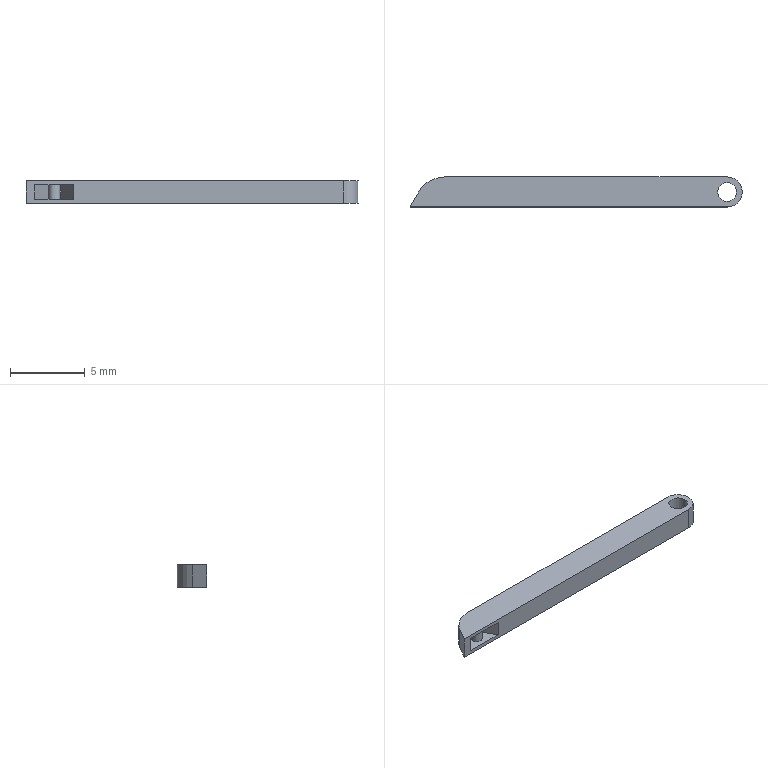Part | SolidWorks | features Extrusion 1, Fillet 1, ICE 1 | 1 solid | 16 faces | box 22.155 x 2 x 1.5 mm | volume 59.83 mm3 | plane 10 | cylinder 6 | commonest cylinder face diameters 0.8 x2 1.25 x2 2 x1 4 x1
STEP:
#1=CARTESIAN_POINT('',(0.3217,-1.25,1.25));
#2=VERTEX_POINT('',#1);
#3=CARTESIAN_POINT('',(1.122,-1.25,1.25));
#4=VERTEX_POINT('',#3);
#5=CARTESIAN_POINT('',(0.7217,-1.25,1.25));
#6=DIRECTION('',(0.,0.,-1.));
#7=DIRECTION('',(-1.,0.,0.));
#8=AXIS2_PLACEMENT_3D('',#5,#6,#7);
#9=CIRCLE('',#8,0.4);
#10=EDGE_CURVE('',#2,#4,#9,.T.);
#11=ORIENTED_EDGE('',*,*,#10,.T.);
#12=CARTESIAN_POINT('',(1.122,-1.25,0.25));
#13=VERTEX_POINT('',#12);
#14=CARTESIAN_POINT('',(1.122,-1.25,1.25));
#15=DIRECTION('',(0.,0.,-1.));
#16=VECTOR('',#15,1000.);
#17=LINE('',#14,#16);
#18=EDGE_CURVE('',#4,#13,#17,.T.);
#19=ORIENTED_EDGE('',*,*,#18,.T.);
#20=CARTESIAN_POINT('',(0.3217,-1.25,0.25));
#21=VERTEX_POINT('',#20);
#22=CARTESIAN_POINT('',(0.7217,-1.25,0.25));
#23=DIRECTION('',(0.,0.,-1.));
#24=DIRECTION('',(-1.,0.,0.));
#25=AXIS2_PLACEMENT_3D('',#22,#23,#24);
#26=CIRCLE('',#25,0.4);
#27=EDGE_CURVE('',#21,#13,#26,.T.);
#28=ORIENTED_EDGE('',*,*,#27,.F.);
#29=CARTESIAN_POINT('',(0.3217,-1.25,1.25));
#30=DIRECTION('',(0.,0.,-1.));
#31=VECTOR('',#30,1000.);
#32=LINE('',#29,#31);
#33=EDGE_CURVE('',#2,#21,#32,.T.);
#34=ORIENTED_EDGE('',*,*,#33,.F.);
#35=EDGE_LOOP('',(#11,#19,#28,#34));
#36=FACE_OUTER_BOUND('',#35,.T.);
#37=CARTESIAN_POINT('',(0.7217,-1.25,1.25));
#38=DIRECTION('',(0.,0.,-1.));
#39=DIRECTION('',(-1.,0.,0.));
#40=AXIS2_PLACEMENT_3D('',#37,#38,#39);
#41=CYLINDRICAL_SURFACE('',#40,0.4);
#42=ADVANCED_FACE('',(#36),#41,.T.);
#43=CARTESIAN_POINT('',(19.375,-1.,1.5));
#44=VERTEX_POINT('',#43);
#45=CARTESIAN_POINT('',(20.625,-1.,1.5));
#46=VERTEX_POINT('',#45);
#47=CARTESIAN_POINT('',(20.,-1.,1.5));
#48=DIRECTION('',(0.,0.,1.));
#49=DIRECTION('',(1.,0.,0.));
#50=AXIS2_PLACEMENT_3D('',#47,#48,#49);
#51=CIRCLE('',#50,0.625);
#52=EDGE_CURVE('',#44,#46,#51,.T.);
#53=ORIENTED_EDGE('',*,*,#52,.T.);
#54=CARTESIAN_POINT('',(20.625,-1.,0.));
#55=VERTEX_POINT('',#54);
#56=CARTESIAN_POINT('',(20.625,-1.,1.5));
#57=DIRECTION('',(0.,0.,-1.));
#58=VECTOR('',#57,1000.);
#59=LINE('',#56,#58);
#60=EDGE_CURVE('',#46,#55,#59,.T.);
#61=ORIENTED_EDGE('',*,*,#60,.T.);
#62=CARTESIAN_POINT('',(19.375,-1.,0.));
#63=VERTEX_POINT('',#62);
#64=CARTESIAN_POINT('',(20.,-1.,0.));
#65=DIRECTION('',(0.,0.,1.));
#66=DIRECTION('',(1.,0.,0.));
#67=AXIS2_PLACEMENT_3D('',#64,#65,#66);
#68=CIRCLE('',#67,0.625);
#69=EDGE_CURVE('',#63,#55,#68,.T.);
#70=ORIENTED_EDGE('',*,*,#69,.F.);
#71=CARTESIAN_POINT('',(19.375,-1.,1.5));
#72=DIRECTION('',(0.,0.,-1.));
#73=VECTOR('',#72,1000.);
#74=LINE('',#71,#73);
#75=EDGE_CURVE('',#44,#63,#74,.T.);
#76=ORIENTED_EDGE('',*,*,#75,.F.);
#77=EDGE_LOOP('',(#53,#61,#70,#76));
#78=FACE_OUTER_BOUND('',#77,.T.);
#79=CARTESIAN_POINT('',(20.,-1.,1.5));
#80=DIRECTION('',(0.,0.,-1.));
#81=DIRECTION('',(-1.,0.,0.));
#82=AXIS2_PLACEMENT_3D('',#79,#80,#81);
#83=CYLINDRICAL_SURFACE('',#82,0.625);
#84=ADVANCED_FACE('',(#78),#83,.F.);
#85=CARTESIAN_POINT('',(-1.155,-2.,0.));
#86=VERTEX_POINT('',#85);
#87=CARTESIAN_POINT('',(20.,-2.,0.));
#88=VERTEX_POINT('',#87);
#89=CARTESIAN_POINT('',(20.,-2.,0.));
#90=DIRECTION('',(1.,0.,0.));
#91=VECTOR('',#90,1000.);
#92=LINE('',#89,#91);
#93=EDGE_CURVE('',#86,#88,#92,.T.);
#94=ORIENTED_EDGE('',*,*,#93,.T.);
#95=CARTESIAN_POINT('',(20.,-2.,1.5));
#96=VERTEX_POINT('',#95);
#97=CARTESIAN_POINT('',(20.,-2.,1.5));
#98=DIRECTION('',(0.,0.,-1.));
#99=VECTOR('',#98,1000.);
#100=LINE('',#97,#99);
#101=EDGE_CURVE('',#96,#88,#100,.T.);
#102=ORIENTED_EDGE('',*,*,#101,.F.);
#103=CARTESIAN_POINT('',(-1.155,-2.,1.5));
#104=VERTEX_POINT('',#103);
#105=CARTESIAN_POINT('',(20.,-2.,1.5));
#106=DIRECTION('',(1.,0.,0.));
#107=VECTOR('',#106,1000.);
#108=LINE('',#105,#107);
#109=EDGE_CURVE('',#104,#96,#108,.T.);
#110=ORIENTED_EDGE('',*,*,#109,.F.);
#111=CARTESIAN_POINT('',(-1.155,-2.,1.5));
#112=DIRECTION('',(0.,0.,-1.));
#113=VECTOR('',#112,1000.);
#114=LINE('',#111,#113);
#115=EDGE_CURVE('',#104,#86,#114,.T.);
#116=ORIENTED_EDGE('',*,*,#115,.T.);
#117=EDGE_LOOP('',(#94,#102,#110,#116));
#118=FACE_OUTER_BOUND('',#117,.T.);
#119=CARTESIAN_POINT('',(2.021,-2.,1.25));
#120=VERTEX_POINT('',#119);
#121=CARTESIAN_POINT('',(-0.5774,-2.,1.25));
#122=VERTEX_POINT('',#121);
#123=CARTESIAN_POINT('',(0.,-2.,1.25));
#124=DIRECTION('',(-1.,0.,0.));
#125=VECTOR('',#124,1000.);
#126=LINE('',#123,#125);
#127=EDGE_CURVE('',#120,#122,#126,.T.);
#128=ORIENTED_EDGE('',*,*,#127,.F.);
#129=CARTESIAN_POINT('',(2.021,-2.,0.25));
#130=VERTEX_POINT('',#129);
#131=CARTESIAN_POINT('',(2.021,-2.,1.25));
#132=DIRECTION('',(0.,0.,-1.));
#133=VECTOR('',#132,1000.);
#134=LINE('',#131,#133);
#135=EDGE_CURVE('',#120,#130,#134,.T.);
#136=ORIENTED_EDGE('',*,*,#135,.T.);
#137=CARTESIAN_POINT('',(-0.5774,-2.,0.25));
#138=VERTEX_POINT('',#137);
#139=CARTESIAN_POINT('',(0.,-2.,0.25));
#140=DIRECTION('',(-1.,0.,0.));
#141=VECTOR('',#140,1000.);
#142=LINE('',#139,#141);
#143=EDGE_CURVE('',#130,#138,#142,.T.);
#144=ORIENTED_EDGE('',*,*,#143,.T.);
#145=CARTESIAN_POINT('',(-0.5774,-2.,1.25));
#146=DIRECTION('',(0.,0.,-1.));
#147=VECTOR('',#146,1000.);
#148=LINE('',#145,#147);
#149=EDGE_CURVE('',#122,#138,#148,.T.);
#150=ORIENTED_EDGE('',*,*,#149,.F.);
#151=EDGE_LOOP('',(#128,#136,#144,#150));
#152=FACE_BOUND('',#151,.T.);
#153=CARTESIAN_POINT('',(20.,-2.,1.5));
#154=DIRECTION('',(0.,1.,0.));
#155=DIRECTION('',(-1.,0.,0.));
#156=AXIS2_PLACEMENT_3D('',#153,#154,#155);
#157=PLANE('',#156);
#158=ADVANCED_FACE('',(#118,#152),#157,.F.);
#159=CARTESIAN_POINT('',(20.,0.,1.5));
#160=VERTEX_POINT('',#159);
#161=CARTESIAN_POINT('',(1.155,0.,1.5));
#162=VERTEX_POINT('',#161);
#163=CARTESIAN_POINT('',(0.,0.,1.5));
#164=DIRECTION('',(-1.,0.,0.));
#165=VECTOR('',#164,1000.);
#166=LINE('',#163,#165);
#167=EDGE_CURVE('',#160,#162,#166,.T.);
#168=ORIENTED_EDGE('',*,*,#167,.T.);
#169=CARTESIAN_POINT('',(-0.5774,-1.,1.5));
#170=VERTEX_POINT('',#169);
#171=CARTESIAN_POINT('',(1.155,-2.,1.5));
#172=DIRECTION('',(0.,0.,1.));
#173=DIRECTION('',(-1.,0.,0.));
#174=AXIS2_PLACEMENT_3D('',#171,#172,#173);
#175=CIRCLE('',#174,2.);
#176=EDGE_CURVE('',#162,#170,#175,.T.);
#177=ORIENTED_EDGE('',*,*,#176,.T.);
#178=CARTESIAN_POINT('',(-1.155,-2.,1.5));
#179=DIRECTION('',(-0.5,-0.866,0.));
#180=VECTOR('',#179,1000.);
#181=LINE('',#178,#180);
#182=EDGE_CURVE('',#170,#104,#181,.T.);
#183=ORIENTED_EDGE('',*,*,#182,.T.);
#184=ORIENTED_EDGE('',*,*,#109,.T.);
#185=CARTESIAN_POINT('',(20.,-1.,1.5));
#186=DIRECTION('',(0.,0.,1.));
#187=DIRECTION('',(-1.,0.,0.));
#188=AXIS2_PLACEMENT_3D('',#185,#186,#187);
#189=CIRCLE('',#188,1.);
#190=EDGE_CURVE('',#96,#160,#189,.T.);
#191=ORIENTED_EDGE('',*,*,#190,.T.);
#192=EDGE_LOOP('',(#168,#177,#183,#184,#191));
#193=FACE_OUTER_BOUND('',#192,.T.);
#194=ORIENTED_EDGE('',*,*,#52,.F.);
#195=CARTESIAN_POINT('',(20.,-1.,1.5));
#196=DIRECTION('',(0.,0.,1.));
#197=DIRECTION('',(1.,0.,0.));
#198=AXIS2_PLACEMENT_3D('',#195,#196,#197);
#199=CIRCLE('',#198,0.625);
#200=EDGE_CURVE('',#46,#44,#199,.T.);
#201=ORIENTED_EDGE('',*,*,#200,.F.);
#202=EDGE_LOOP('',(#194,#201));
#203=FACE_BOUND('',#202,.T.);
#204=CARTESIAN_POINT('',(20.,-1.,1.5));
#205=DIRECTION('',(0.,0.,-1.));
#206=DIRECTION('',(-1.,0.,0.));
#207=AXIS2_PLACEMENT_3D('',#204,#205,#206);
#208=PLANE('',#207);
#209=ADVANCED_FACE('',(#193,#203),#208,.F.);
#210=CARTESIAN_POINT('',(-0.5774,-1.,0.));
#211=VERTEX_POINT('',#210);
#212=CARTESIAN_POINT('',(-1.155,-2.,0.));
#213=DIRECTION('',(-0.5,-0.866,0.));
#214=VECTOR('',#213,1000.);
#215=LINE('',#212,#214);
#216=EDGE_CURVE('',#211,#86,#215,.T.);
#217=ORIENTED_EDGE('',*,*,#216,.F.);
#218=CARTESIAN_POINT('',(1.155,0.,0.));
#219=VERTEX_POINT('',#218);
#220=CARTESIAN_POINT('',(1.155,-2.,0.));
#221=DIRECTION('',(0.,0.,-1.));
#222=DIRECTION('',(-1.,0.,0.));
#223=AXIS2_PLACEMENT_3D('',#220,#221,#222);
#224=CIRCLE('',#223,2.);
#225=EDGE_CURVE('',#211,#219,#224,.T.);
#226=ORIENTED_EDGE('',*,*,#225,.T.);
#227=CARTESIAN_POINT('',(20.,0.,0.));
#228=VERTEX_POINT('',#227);
#229=CARTESIAN_POINT('',(0.,0.,0.));
#230=DIRECTION('',(-1.,0.,0.));
#231=VECTOR('',#230,1000.);
#232=LINE('',#229,#231);
#233=EDGE_CURVE('',#228,#219,#232,.T.);
#234=ORIENTED_EDGE('',*,*,#233,.F.);
#235=CARTESIAN_POINT('',(20.,-1.,0.));
#236=DIRECTION('',(0.,0.,1.));
#237=DIRECTION('',(-1.,0.,0.));
#238=AXIS2_PLACEMENT_3D('',#235,#236,#237);
#239=CIRCLE('',#238,1.);
#240=EDGE_CURVE('',#88,#228,#239,.T.);
#241=ORIENTED_EDGE('',*,*,#240,.F.);
#242=ORIENTED_EDGE('',*,*,#93,.F.);
#243=EDGE_LOOP('',(#217,#226,#234,#241,#242));
#244=FACE_OUTER_BOUND('',#243,.T.);
#245=ORIENTED_EDGE('',*,*,#69,.T.);
#246=CARTESIAN_POINT('',(20.,-1.,0.));
#247=DIRECTION('',(0.,0.,1.));
#248=DIRECTION('',(1.,0.,0.));
#249=AXIS2_PLACEMENT_3D('',#246,#247,#248);
#250=CIRCLE('',#249,0.625);
#251=EDGE_CURVE('',#55,#63,#250,.T.);
#252=ORIENTED_EDGE('',*,*,#251,.T.);
#253=EDGE_LOOP('',(#245,#252));
#254=FACE_BOUND('',#253,.T.);
#255=CARTESIAN_POINT('',(20.,-1.,0.));
#256=DIRECTION('',(0.,0.,-1.));
#257=DIRECTION('',(-1.,0.,0.));
#258=AXIS2_PLACEMENT_3D('',#255,#256,#257);
#259=PLANE('',#258);
#260=ADVANCED_FACE('',(#244,#254),#259,.T.);
#261=ORIENTED_EDGE('',*,*,#182,.F.);
#262=CARTESIAN_POINT('',(-0.5774,-1.,1.5));
#263=DIRECTION('',(0.,0.,-1.));
#264=VECTOR('',#263,1000.);
#265=LINE('',#262,#264);
#266=EDGE_CURVE('',#170,#211,#265,.T.);
#267=ORIENTED_EDGE('',*,*,#266,.T.);
#268=ORIENTED_EDGE('',*,*,#216,.T.);
#269=ORIENTED_EDGE('',*,*,#115,.F.);
#270=EDGE_LOOP('',(#261,#267,#268,#269));
#271=FACE_OUTER_BOUND('',#270,.T.);
#272=CARTESIAN_POINT('',(-1.155,-2.,1.5));
#273=DIRECTION('',(0.866,-0.5,0.));
#274=DIRECTION('',(0.5,0.866,0.));
#275=AXIS2_PLACEMENT_3D('',#272,#273,#274);
#276=PLANE('',#275);
#277=ADVANCED_FACE('',(#271),#276,.F.);
#278=ORIENTED_EDGE('',*,*,#240,.T.);
#279=CARTESIAN_POINT('',(20.,0.,1.5));
#280=DIRECTION('',(0.,0.,-1.));
#281=VECTOR('',#280,1000.);
#282=LINE('',#279,#281);
#283=EDGE_CURVE('',#160,#228,#282,.T.);
#284=ORIENTED_EDGE('',*,*,#283,.F.);
#285=ORIENTED_EDGE('',*,*,#190,.F.);
#286=ORIENTED_EDGE('',*,*,#101,.T.);
#287=EDGE_LOOP('',(#278,#284,#285,#286));
#288=FACE_OUTER_BOUND('',#287,.T.);
#289=CARTESIAN_POINT('',(20.,-1.,1.5));
#290=DIRECTION('',(0.,0.,-1.));
#291=DIRECTION('',(-1.,0.,0.));
#292=AXIS2_PLACEMENT_3D('',#289,#290,#291);
#293=CYLINDRICAL_SURFACE('',#292,1.);
#294=ADVANCED_FACE('',(#288),#293,.T.);
#295=ORIENTED_EDGE('',*,*,#233,.T.);
#296=CARTESIAN_POINT('',(1.155,0.,1.5));
#297=DIRECTION('',(0.,0.,1.));
#298=VECTOR('',#297,1000.);
#299=LINE('',#296,#298);
#300=EDGE_CURVE('',#219,#162,#299,.T.);
#301=ORIENTED_EDGE('',*,*,#300,.T.);
#302=ORIENTED_EDGE('',*,*,#167,.F.);
#303=ORIENTED_EDGE('',*,*,#283,.T.);
#304=EDGE_LOOP('',(#295,#301,#302,#303));
#305=FACE_OUTER_BOUND('',#304,.T.);
#306=CARTESIAN_POINT('',(0.,0.,1.5));
#307=DIRECTION('',(0.,-1.,0.));
#308=DIRECTION('',(1.,0.,0.));
#309=AXIS2_PLACEMENT_3D('',#306,#307,#308);
#310=PLANE('',#309);
#311=ADVANCED_FACE('',(#305),#310,.F.);
#312=ORIENTED_EDGE('',*,*,#60,.F.);
#313=ORIENTED_EDGE('',*,*,#200,.T.);
#314=ORIENTED_EDGE('',*,*,#75,.T.);
#315=ORIENTED_EDGE('',*,*,#251,.F.);
#316=EDGE_LOOP('',(#312,#313,#314,#315));
#317=FACE_OUTER_BOUND('',#316,.T.);
#318=CARTESIAN_POINT('',(20.,-1.,1.5));
#319=DIRECTION('',(0.,0.,-1.));
#320=DIRECTION('',(-1.,0.,0.));
#321=AXIS2_PLACEMENT_3D('',#318,#319,#320);
#322=CYLINDRICAL_SURFACE('',#321,0.625);
#323=ADVANCED_FACE('',(#317),#322,.F.);
#324=CARTESIAN_POINT('',(1.155,-0.5,0.25));
#325=VERTEX_POINT('',#324);
#326=CARTESIAN_POINT('',(0.6495,0.375,0.25));
#327=DIRECTION('',(0.5,-0.866,0.));
#328=VECTOR('',#327,1000.);
#329=LINE('',#326,#328);
#330=EDGE_CURVE('',#325,#130,#329,.T.);
#331=ORIENTED_EDGE('',*,*,#330,.T.);
#332=ORIENTED_EDGE('',*,*,#135,.F.);
#333=CARTESIAN_POINT('',(1.155,-0.5,1.25));
#334=VERTEX_POINT('',#333);
#335=CARTESIAN_POINT('',(0.6495,0.375,1.25));
#336=DIRECTION('',(0.5,-0.866,0.));
#337=VECTOR('',#336,1000.);
#338=LINE('',#335,#337);
#339=EDGE_CURVE('',#334,#120,#338,.T.);
#340=ORIENTED_EDGE('',*,*,#339,.F.);
#341=CARTESIAN_POINT('',(1.155,-0.5,1.25));
#342=DIRECTION('',(0.,0.,-1.));
#343=VECTOR('',#342,1000.);
#344=LINE('',#341,#343);
#345=EDGE_CURVE('',#334,#325,#344,.T.);
#346=ORIENTED_EDGE('',*,*,#345,.T.);
#347=EDGE_LOOP('',(#331,#332,#340,#346));
#348=FACE_OUTER_BOUND('',#347,.T.);
#349=CARTESIAN_POINT('',(0.6495,0.375,1.25));
#350=DIRECTION('',(0.866,0.5,0.));
#351=DIRECTION('',(-0.5,0.866,0.));
#352=AXIS2_PLACEMENT_3D('',#349,#350,#351);
#353=PLANE('',#352);
#354=ADVANCED_FACE('',(#348),#353,.F.);
#355=CARTESIAN_POINT('',(0.2887,-0.5,0.25));
#356=VERTEX_POINT('',#355);
#357=CARTESIAN_POINT('',(0.,-0.5,0.25));
#358=DIRECTION('',(1.,0.,0.));
#359=VECTOR('',#358,1000.);
#360=LINE('',#357,#359);
#361=EDGE_CURVE('',#356,#325,#360,.T.);
#362=ORIENTED_EDGE('',*,*,#361,.T.);
#363=ORIENTED_EDGE('',*,*,#345,.F.);
#364=CARTESIAN_POINT('',(0.2887,-0.5,1.25));
#365=VERTEX_POINT('',#364);
#366=CARTESIAN_POINT('',(0.,-0.5,1.25));
#367=DIRECTION('',(1.,0.,0.));
#368=VECTOR('',#367,1000.);
#369=LINE('',#366,#368);
#370=EDGE_CURVE('',#365,#334,#369,.T.);
#371=ORIENTED_EDGE('',*,*,#370,.F.);
#372=CARTESIAN_POINT('',(0.2887,-0.5,1.25));
#373=DIRECTION('',(0.,0.,-1.));
#374=VECTOR('',#373,1000.);
#375=LINE('',#372,#374);
#376=EDGE_CURVE('',#365,#356,#375,.T.);
#377=ORIENTED_EDGE('',*,*,#376,.T.);
#378=EDGE_LOOP('',(#362,#363,#371,#377));
#379=FACE_OUTER_BOUND('',#378,.T.);
#380=CARTESIAN_POINT('',(0.,-0.5,1.25));
#381=DIRECTION('',(0.,1.,0.));
#382=DIRECTION('',(-1.,0.,0.));
#383=AXIS2_PLACEMENT_3D('',#380,#381,#382);
#384=PLANE('',#383);
#385=ADVANCED_FACE('',(#379),#384,.F.);
#386=CARTESIAN_POINT('',(0.433,-0.25,0.25));
#387=DIRECTION('',(0.5,0.866,0.));
#388=VECTOR('',#387,1000.);
#389=LINE('',#386,#388);
#390=EDGE_CURVE('',#138,#356,#389,.T.);
#391=ORIENTED_EDGE('',*,*,#390,.T.);
#392=ORIENTED_EDGE('',*,*,#376,.F.);
#393=CARTESIAN_POINT('',(0.433,-0.25,1.25));
#394=DIRECTION('',(0.5,0.866,0.));
#395=VECTOR('',#394,1000.);
#396=LINE('',#393,#395);
#397=EDGE_CURVE('',#122,#365,#396,.T.);
#398=ORIENTED_EDGE('',*,*,#397,.F.);
#399=ORIENTED_EDGE('',*,*,#149,.T.);
#400=EDGE_LOOP('',(#391,#392,#398,#399));
#401=FACE_OUTER_BOUND('',#400,.T.);
#402=CARTESIAN_POINT('',(0.433,-0.25,1.25));
#403=DIRECTION('',(-0.866,0.5,0.));
#404=DIRECTION('',(-0.5,-0.866,0.));
#405=AXIS2_PLACEMENT_3D('',#402,#403,#404);
#406=PLANE('',#405);
#407=ADVANCED_FACE('',(#401),#406,.F.);
#408=ORIENTED_EDGE('',*,*,#18,.F.);
#409=CARTESIAN_POINT('',(0.7217,-1.25,1.25));
#410=DIRECTION('',(0.,0.,-1.));
#411=DIRECTION('',(-1.,0.,0.));
#412=AXIS2_PLACEMENT_3D('',#409,#410,#411);
#413=CIRCLE('',#412,0.4);
#414=EDGE_CURVE('',#4,#2,#413,.T.);
#415=ORIENTED_EDGE('',*,*,#414,.T.);
#416=ORIENTED_EDGE('',*,*,#33,.T.);
#417=CARTESIAN_POINT('',(0.7217,-1.25,0.25));
#418=DIRECTION('',(0.,0.,-1.));
#419=DIRECTION('',(-1.,0.,0.));
#420=AXIS2_PLACEMENT_3D('',#417,#418,#419);
#421=CIRCLE('',#420,0.4);
#422=EDGE_CURVE('',#13,#21,#421,.T.);
#423=ORIENTED_EDGE('',*,*,#422,.F.);
#424=EDGE_LOOP('',(#408,#415,#416,#423));
#425=FACE_OUTER_BOUND('',#424,.T.);
#426=CARTESIAN_POINT('',(0.7217,-1.25,1.25));
#427=DIRECTION('',(0.,0.,-1.));
#428=DIRECTION('',(-1.,0.,0.));
#429=AXIS2_PLACEMENT_3D('',#426,#427,#428);
#430=CYLINDRICAL_SURFACE('',#429,0.4);
#431=ADVANCED_FACE('',(#425),#430,.T.);
#432=ORIENTED_EDGE('',*,*,#339,.T.);
#433=ORIENTED_EDGE('',*,*,#127,.T.);
#434=ORIENTED_EDGE('',*,*,#397,.T.);
#435=ORIENTED_EDGE('',*,*,#370,.T.);
#436=EDGE_LOOP('',(#432,#433,#434,#435));
#437=FACE_OUTER_BOUND('',#436,.T.);
#438=ORIENTED_EDGE('',*,*,#10,.F.);
#439=ORIENTED_EDGE('',*,*,#414,.F.);
#440=EDGE_LOOP('',(#438,#439));
#441=FACE_BOUND('',#440,.T.);
#442=CARTESIAN_POINT('',(0.,0.,1.25));
#443=DIRECTION('',(0.,0.,-1.));
#444=DIRECTION('',(-1.,0.,0.));
#445=AXIS2_PLACEMENT_3D('',#442,#443,#444);
#446=PLANE('',#445);
#447=ADVANCED_FACE('',(#437,#441),#446,.T.);
#448=ORIENTED_EDGE('',*,*,#330,.F.);
#449=ORIENTED_EDGE('',*,*,#361,.F.);
#450=ORIENTED_EDGE('',*,*,#390,.F.);
#451=ORIENTED_EDGE('',*,*,#143,.F.);
#452=EDGE_LOOP('',(#448,#449,#450,#451));
#453=FACE_OUTER_BOUND('',#452,.T.);
#454=ORIENTED_EDGE('',*,*,#27,.T.);
#455=ORIENTED_EDGE('',*,*,#422,.T.);
#456=EDGE_LOOP('',(#454,#455));
#457=FACE_BOUND('',#456,.T.);
#458=CARTESIAN_POINT('',(0.,0.,0.25));
#459=DIRECTION('',(0.,0.,-1.));
#460=DIRECTION('',(-1.,0.,0.));
#461=AXIS2_PLACEMENT_3D('',#458,#459,#460);
#462=PLANE('',#461);
#463=ADVANCED_FACE('',(#453,#457),#462,.F.);
#464=ORIENTED_EDGE('',*,*,#176,.F.);
#465=ORIENTED_EDGE('',*,*,#300,.F.);
#466=ORIENTED_EDGE('',*,*,#225,.F.);
#467=ORIENTED_EDGE('',*,*,#266,.F.);
#468=EDGE_LOOP('',(#464,#465,#466,#467));
#469=FACE_OUTER_BOUND('',#468,.T.);
#470=CARTESIAN_POINT('',(1.155,-2.,1.5));
#471=DIRECTION('',(0.,0.,-1.));
#472=DIRECTION('',(-1.,0.,0.));
#473=AXIS2_PLACEMENT_3D('',#470,#471,#472);
#474=CYLINDRICAL_SURFACE('',#473,2.);
#475=ADVANCED_FACE('',(#469),#474,.T.);
#476=CLOSED_SHELL('',(#42,#84,#158,#209,#260,#277,#294,#311,#323,#354,#385,#407,#431,#447,#463,#475));
#477=MANIFOLD_SOLID_BREP('',#476);
#478=CARTESIAN_POINT('',(0.,0.,0.));
#479=DIRECTION('',(0.,0.,1.));
#480=DIRECTION('',(1.,0.,0.));
#481=AXIS2_PLACEMENT_3D('',#478,#479,#480);
#482=(LENGTH_UNIT()NAMED_UNIT(*)SI_UNIT(.MILLI.,.METRE.));
#483=UNCERTAINTY_MEASURE_WITH_UNIT(LENGTH_MEASURE(0.00001),#482,'','');
#484=(NAMED_UNIT(*)PLANE_ANGLE_UNIT()SI_UNIT($,.RADIAN.));
#485=(NAMED_UNIT(*)SI_UNIT($,.STERADIAN.)SOLID_ANGLE_UNIT());
#486=(GEOMETRIC_REPRESENTATION_CONTEXT(3)GLOBAL_UNCERTAINTY_ASSIGNED_CONTEXT((#483))GLOBAL_UNIT_ASSIGNED_CONTEXT((#482,#484,#485))REPRESENTATION_CONTEXT('',''));
#487=ADVANCED_BREP_SHAPE_REPRESENTATION('',(#477,#481),#486);